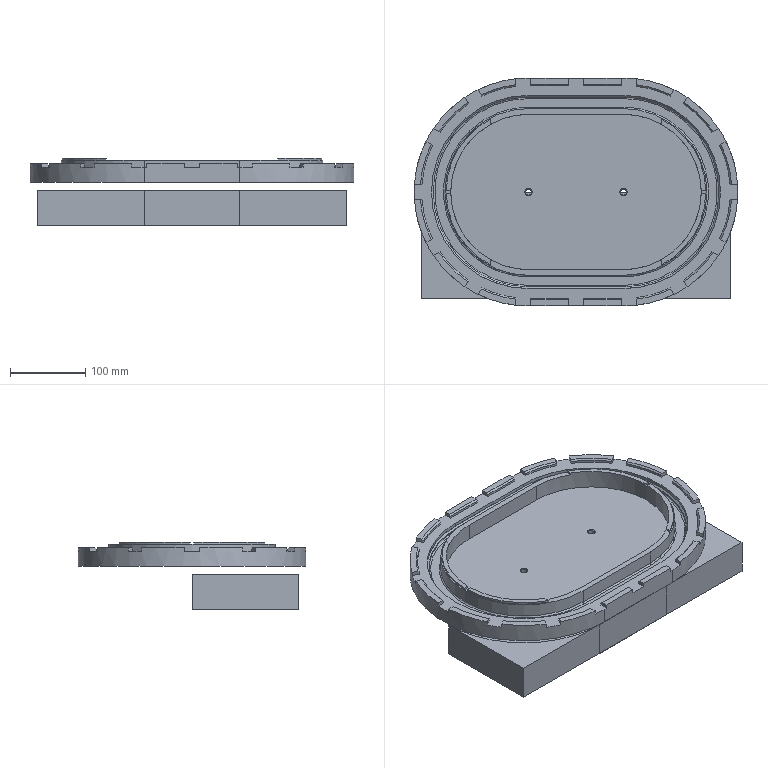Part | 3 solids | 186 faces | box 429 x 302 x 89.371 mm | volume 4375046 mm3 | plane 104 | cylinder 46 | cone 24 | torus 12 | commonest cylinder face diameters 282 x12 0.4 x5 4 x5 218 x4 8 x2 206 x2